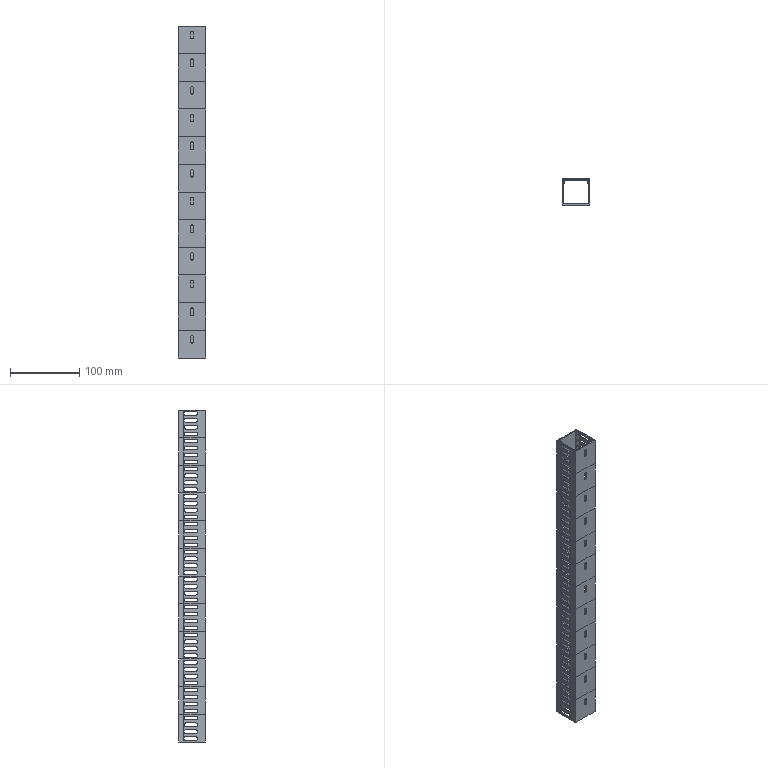Part | STEP file | 23 solids | 2003 faces | box 40 x 38.5 x 480 mm | volume 109641 mm3 | plane 1032 | cylinder 971 | commonest cylinder face diameters 5 x323 1 x204 2 x180 24 x144 26 x120